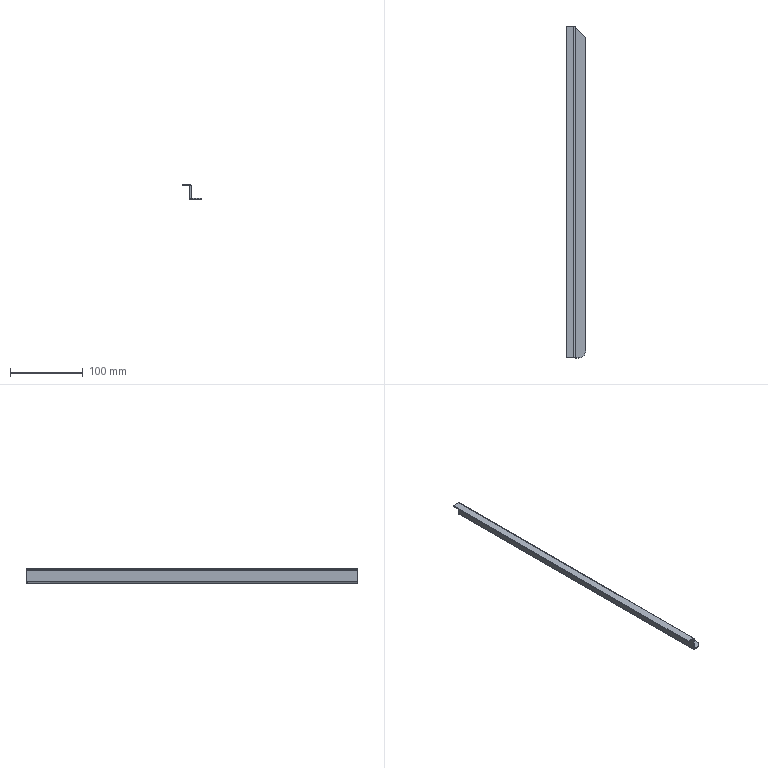Part | STEP file | Left Side Panel Frame Right | 1 solid | 21 faces | box 26.5 x 455 x 20 mm | volume 29759 mm3 | plane 14 | cylinder 7 | commonest cylinder face diameters 0.15 x2 1 x2 4 x2 20 x1
STEP:
#1=CARTESIAN_POINT('',(0.,30.962,817.654));
#2=VERTEX_POINT('',#1);
#3=CARTESIAN_POINT('',(0.,31.037,817.579));
#4=VERTEX_POINT('',#3);
#5=CARTESIAN_POINT('',(0.,30.962,817.579));
#6=DIRECTION('',(-1.,0.,0.));
#7=DIRECTION('',(0.,0.,1.));
#8=AXIS2_PLACEMENT_3D('',#5,#6,#7);
#9=CIRCLE('',#8,0.075);
#10=EDGE_CURVE('',#2,#4,#9,.T.);
#11=ORIENTED_EDGE('',*,*,#10,.F.);
#12=CARTESIAN_POINT('',(-1.5,30.962,817.654));
#13=VERTEX_POINT('',#12);
#14=CARTESIAN_POINT('',(0.,30.962,817.654));
#15=DIRECTION('',(-1.,0.,0.));
#16=VECTOR('',#15,1000.);
#17=LINE('',#14,#16);
#18=EDGE_CURVE('',#2,#13,#17,.T.);
#19=ORIENTED_EDGE('',*,*,#18,.T.);
#20=CARTESIAN_POINT('',(-1.5,31.037,817.579));
#21=VERTEX_POINT('',#20);
#22=CARTESIAN_POINT('',(-1.5,30.962,817.579));
#23=DIRECTION('',(1.,0.,0.));
#24=DIRECTION('',(0.,0.,1.));
#25=AXIS2_PLACEMENT_3D('',#22,#23,#24);
#26=CIRCLE('',#25,0.075);
#27=EDGE_CURVE('',#21,#13,#26,.T.);
#28=ORIENTED_EDGE('',*,*,#27,.F.);
#29=CARTESIAN_POINT('',(0.,31.037,817.579));
#30=DIRECTION('',(-1.,0.,0.));
#31=VECTOR('',#30,1000.);
#32=LINE('',#29,#31);
#33=EDGE_CURVE('',#4,#21,#32,.T.);
#34=ORIENTED_EDGE('',*,*,#33,.F.);
#35=EDGE_LOOP('',(#11,#19,#28,#34));
#36=FACE_OUTER_BOUND('',#35,.T.);
#37=CARTESIAN_POINT('',(0.,30.962,817.579));
#38=DIRECTION('',(-1.,0.,0.));
#39=DIRECTION('',(0.,0.,1.));
#40=AXIS2_PLACEMENT_3D('',#37,#38,#39);
#41=CYLINDRICAL_SURFACE('',#40,0.075);
#42=ADVANCED_FACE('',(#36),#41,.F.);
#43=CARTESIAN_POINT('',(-1.5,30.887,817.429));
#44=VERTEX_POINT('',#43);
#45=CARTESIAN_POINT('',(-1.5,30.887,817.579));
#46=VERTEX_POINT('',#45);
#47=CARTESIAN_POINT('',(-1.5,30.887,817.579));
#48=DIRECTION('',(0.,0.,1.));
#49=VECTOR('',#48,1000.);
#50=LINE('',#47,#49);
#51=EDGE_CURVE('',#44,#46,#50,.T.);
#52=ORIENTED_EDGE('',*,*,#51,.F.);
#53=CARTESIAN_POINT('',(-1.5,-422.413,817.429));
#54=VERTEX_POINT('',#53);
#55=CARTESIAN_POINT('',(-1.5,0.,817.429));
#56=DIRECTION('',(0.,-1.,0.));
#57=VECTOR('',#56,1000.);
#58=LINE('',#55,#57);
#59=EDGE_CURVE('',#44,#54,#58,.T.);
#60=ORIENTED_EDGE('',*,*,#59,.T.);
#61=CARTESIAN_POINT('',(-1.5,-422.413,833.429));
#62=VERTEX_POINT('',#61);
#63=CARTESIAN_POINT('',(-1.5,-422.413,0.));
#64=DIRECTION('',(0.,0.,1.));
#65=VECTOR('',#64,1000.);
#66=LINE('',#63,#65);
#67=EDGE_CURVE('',#54,#62,#66,.T.);
#68=ORIENTED_EDGE('',*,*,#67,.T.);
#69=CARTESIAN_POINT('',(-1.5,32.587,833.429));
#70=VERTEX_POINT('',#69);
#71=CARTESIAN_POINT('',(-1.5,0.,833.429));
#72=DIRECTION('',(0.,1.,0.));
#73=VECTOR('',#72,1000.);
#74=LINE('',#71,#73);
#75=EDGE_CURVE('',#62,#70,#74,.T.);
#76=ORIENTED_EDGE('',*,*,#75,.T.);
#77=CARTESIAN_POINT('',(-1.5,32.587,815.429));
#78=VERTEX_POINT('',#77);
#79=CARTESIAN_POINT('',(-1.5,32.587,0.));
#80=DIRECTION('',(0.,0.,-1.));
#81=VECTOR('',#80,1000.);
#82=LINE('',#79,#81);
#83=EDGE_CURVE('',#70,#78,#82,.T.);
#84=ORIENTED_EDGE('',*,*,#83,.T.);
#85=CARTESIAN_POINT('',(-1.5,31.037,815.429));
#86=VERTEX_POINT('',#85);
#87=CARTESIAN_POINT('',(-1.5,0.,815.429));
#88=DIRECTION('',(0.,-1.,0.));
#89=VECTOR('',#88,1000.);
#90=LINE('',#87,#89);
#91=EDGE_CURVE('',#78,#86,#90,.T.);
#92=ORIENTED_EDGE('',*,*,#91,.T.);
#93=CARTESIAN_POINT('',(-1.5,31.037,0.));
#94=DIRECTION('',(0.,0.,1.));
#95=VECTOR('',#94,1000.);
#96=LINE('',#93,#95);
#97=EDGE_CURVE('',#86,#21,#96,.T.);
#98=ORIENTED_EDGE('',*,*,#97,.T.);
#99=ORIENTED_EDGE('',*,*,#27,.T.);
#100=CARTESIAN_POINT('',(-1.5,30.962,817.579));
#101=DIRECTION('',(1.,0.,0.));
#102=DIRECTION('',(0.,0.,1.));
#103=AXIS2_PLACEMENT_3D('',#100,#101,#102);
#104=CIRCLE('',#103,0.075);
#105=EDGE_CURVE('',#13,#46,#104,.T.);
#106=ORIENTED_EDGE('',*,*,#105,.T.);
#107=EDGE_LOOP('',(#52,#60,#68,#76,#84,#92,#98,#99,#106));
#108=FACE_OUTER_BOUND('',#107,.T.);
#109=CARTESIAN_POINT('',(-1.5,0.,0.));
#110=DIRECTION('',(-1.,0.,0.));
#111=DIRECTION('',(0.,0.,1.));
#112=AXIS2_PLACEMENT_3D('',#109,#110,#111);
#113=PLANE('',#112);
#114=ADVANCED_FACE('',(#108),#113,.T.);
#115=CARTESIAN_POINT('',(0.5,-422.413,815.429));
#116=VERTEX_POINT('',#115);
#117=CARTESIAN_POINT('',(0.5,-422.413,817.429));
#118=DIRECTION('',(0.,1.,0.));
#119=DIRECTION('',(0.,0.,1.));
#120=AXIS2_PLACEMENT_3D('',#117,#118,#119);
#121=CIRCLE('',#120,2.);
#122=EDGE_CURVE('',#116,#54,#121,.T.);
#123=ORIENTED_EDGE('',*,*,#122,.T.);
#124=ORIENTED_EDGE('',*,*,#59,.F.);
#125=CARTESIAN_POINT('',(0.2,30.887,815.452));
#126=VERTEX_POINT('',#125);
#127=CARTESIAN_POINT('',(0.5,30.887,817.429));
#128=DIRECTION('',(0.,-1.,0.));
#129=DIRECTION('',(0.,0.,1.));
#130=AXIS2_PLACEMENT_3D('',#127,#128,#129);
#131=CIRCLE('',#130,2.);
#132=EDGE_CURVE('',#44,#126,#131,.T.);
#133=ORIENTED_EDGE('',*,*,#132,.T.);
#134=CARTESIAN_POINT('',(0.5,30.587,815.429));
#135=VERTEX_POINT('',#134);
#136=CARTESIAN_POINT('',(0.2,30.887,815.452));
#137=CARTESIAN_POINT('',(0.2993,30.788,815.437));
#138=CARTESIAN_POINT('',(0.3995,30.687,815.429));
#139=CARTESIAN_POINT('',(0.5,30.587,815.429));
#140=(BOUNDED_CURVE()B_SPLINE_CURVE(3,(#136,#137,#138,#139),.UNSPECIFIED.,.F.,.F.)B_SPLINE_CURVE_WITH_KNOTS((4,4),(1.42,1.571),.UNSPECIFIED.)CURVE()GEOMETRIC_REPRESENTATION_ITEM()RATIONAL_B_SPLINE_CURVE((1.,0.9981,0.9981,1.))REPRESENTATION_ITEM(''));
#141=EDGE_CURVE('',#126,#135,#140,.T.);
#142=ORIENTED_EDGE('',*,*,#141,.T.);
#143=CARTESIAN_POINT('',(0.5,30.887,815.429));
#144=DIRECTION('',(0.,-1.,0.));
#145=VECTOR('',#144,1000.);
#146=LINE('',#143,#145);
#147=EDGE_CURVE('',#135,#116,#146,.T.);
#148=ORIENTED_EDGE('',*,*,#147,.T.);
#149=EDGE_LOOP('',(#123,#124,#133,#142,#148));
#150=FACE_OUTER_BOUND('',#149,.T.);
#151=CARTESIAN_POINT('',(0.5,30.887,817.429));
#152=DIRECTION('',(0.,1.,0.));
#153=DIRECTION('',(0.,0.,1.));
#154=AXIS2_PLACEMENT_3D('',#151,#152,#153);
#155=CYLINDRICAL_SURFACE('',#154,2.);
#156=ADVANCED_FACE('',(#150),#155,.T.);
#157=CARTESIAN_POINT('',(0.,31.037,815.429));
#158=VERTEX_POINT('',#157);
#159=CARTESIAN_POINT('',(0.,31.037,815.429));
#160=DIRECTION('',(0.,0.,1.));
#161=VECTOR('',#160,1000.);
#162=LINE('',#159,#161);
#163=EDGE_CURVE('',#158,#4,#162,.T.);
#164=ORIENTED_EDGE('',*,*,#163,.T.);
#165=ORIENTED_EDGE('',*,*,#33,.T.);
#166=ORIENTED_EDGE('',*,*,#97,.F.);
#167=CARTESIAN_POINT('',(0.,31.037,815.429));
#168=DIRECTION('',(1.,0.,0.));
#169=VECTOR('',#168,1000.);
#170=LINE('',#167,#169);
#171=EDGE_CURVE('',#86,#158,#170,.T.);
#172=ORIENTED_EDGE('',*,*,#171,.T.);
#173=EDGE_LOOP('',(#164,#165,#166,#172));
#174=FACE_OUTER_BOUND('',#173,.T.);
#175=CARTESIAN_POINT('',(0.,31.037,815.429));
#176=DIRECTION('',(0.,-1.,0.));
#177=DIRECTION('',(0.,0.,-1.));
#178=AXIS2_PLACEMENT_3D('',#175,#176,#177);
#179=PLANE('',#178);
#180=ADVANCED_FACE('',(#174),#179,.T.);
#181=ORIENTED_EDGE('',*,*,#91,.F.);
#182=CARTESIAN_POINT('',(0.,32.587,815.429));
#183=VERTEX_POINT('',#182);
#184=CARTESIAN_POINT('',(-1.5,32.587,815.429));
#185=DIRECTION('',(1.,0.,0.));
#186=VECTOR('',#185,1000.);
#187=LINE('',#184,#186);
#188=EDGE_CURVE('',#78,#183,#187,.T.);
#189=ORIENTED_EDGE('',*,*,#188,.T.);
#190=CARTESIAN_POINT('',(0.,32.587,815.429));
#191=DIRECTION('',(0.,-1.,0.));
#192=VECTOR('',#191,1000.);
#193=LINE('',#190,#192);
#194=EDGE_CURVE('',#183,#158,#193,.T.);
#195=ORIENTED_EDGE('',*,*,#194,.T.);
#196=ORIENTED_EDGE('',*,*,#171,.F.);
#197=EDGE_LOOP('',(#181,#189,#195,#196));
#198=FACE_OUTER_BOUND('',#197,.T.);
#199=CARTESIAN_POINT('',(-1.5,32.587,815.429));
#200=DIRECTION('',(0.,0.,-1.));
#201=DIRECTION('',(0.,1.,0.));
#202=AXIS2_PLACEMENT_3D('',#199,#200,#201);
#203=PLANE('',#202);
#204=ADVANCED_FACE('',(#198),#203,.T.);
#205=CARTESIAN_POINT('',(0.,32.587,833.429));
#206=VERTEX_POINT('',#205);
#207=CARTESIAN_POINT('',(0.,32.587,835.429));
#208=DIRECTION('',(0.,0.,-1.));
#209=VECTOR('',#208,1000.);
#210=LINE('',#207,#209);
#211=EDGE_CURVE('',#206,#183,#210,.T.);
#212=ORIENTED_EDGE('',*,*,#211,.T.);
#213=ORIENTED_EDGE('',*,*,#188,.F.);
#214=ORIENTED_EDGE('',*,*,#83,.F.);
#215=CARTESIAN_POINT('',(-2.,32.587,833.929));
#216=VERTEX_POINT('',#215);
#217=CARTESIAN_POINT('',(-2.,32.587,833.429));
#218=DIRECTION('',(0.,1.,0.));
#219=DIRECTION('',(0.,0.,1.));
#220=AXIS2_PLACEMENT_3D('',#217,#218,#219);
#221=CIRCLE('',#220,0.5);
#222=EDGE_CURVE('',#216,#70,#221,.T.);
#223=ORIENTED_EDGE('',*,*,#222,.F.);
#224=CARTESIAN_POINT('',(-12.,32.587,833.929));
#225=VERTEX_POINT('',#224);
#226=CARTESIAN_POINT('',(0.,32.587,833.929));
#227=DIRECTION('',(1.,0.,0.));
#228=VECTOR('',#227,1000.);
#229=LINE('',#226,#228);
#230=EDGE_CURVE('',#225,#216,#229,.T.);
#231=ORIENTED_EDGE('',*,*,#230,.F.);
#232=CARTESIAN_POINT('',(-12.,32.587,835.429));
#233=VERTEX_POINT('',#232);
#234=CARTESIAN_POINT('',(-12.,32.587,835.429));
#235=DIRECTION('',(0.,0.,1.));
#236=VECTOR('',#235,1000.);
#237=LINE('',#234,#236);
#238=EDGE_CURVE('',#225,#233,#237,.T.);
#239=ORIENTED_EDGE('',*,*,#238,.T.);
#240=CARTESIAN_POINT('',(-2.,32.587,835.429));
#241=VERTEX_POINT('',#240);
#242=CARTESIAN_POINT('',(-12.,32.587,835.429));
#243=DIRECTION('',(-1.,0.,0.));
#244=VECTOR('',#243,1000.);
#245=LINE('',#242,#244);
#246=EDGE_CURVE('',#241,#233,#245,.T.);
#247=ORIENTED_EDGE('',*,*,#246,.F.);
#248=CARTESIAN_POINT('',(-2.,32.587,833.429));
#249=DIRECTION('',(0.,-1.,0.));
#250=DIRECTION('',(0.,0.,1.));
#251=AXIS2_PLACEMENT_3D('',#248,#249,#250);
#252=CIRCLE('',#251,2.);
#253=EDGE_CURVE('',#206,#241,#252,.T.);
#254=ORIENTED_EDGE('',*,*,#253,.F.);
#255=EDGE_LOOP('',(#212,#213,#214,#223,#231,#239,#247,#254));
#256=FACE_OUTER_BOUND('',#255,.T.);
#257=CARTESIAN_POINT('',(-1.5,32.587,835.429));
#258=DIRECTION('',(0.,1.,0.));
#259=DIRECTION('',(0.,0.,1.));
#260=AXIS2_PLACEMENT_3D('',#257,#258,#259);
#261=PLANE('',#260);
#262=ADVANCED_FACE('',(#256),#261,.T.);
#263=CARTESIAN_POINT('',(-2.,-422.413,833.929));
#264=VERTEX_POINT('',#263);
#265=CARTESIAN_POINT('',(-2.,-422.413,833.429));
#266=DIRECTION('',(0.,1.,0.));
#267=DIRECTION('',(0.,0.,1.));
#268=AXIS2_PLACEMENT_3D('',#265,#266,#267);
#269=CIRCLE('',#268,0.5);
#270=EDGE_CURVE('',#264,#62,#269,.T.);
#271=ORIENTED_EDGE('',*,*,#270,.F.);
#272=CARTESIAN_POINT('',(-2.,32.587,833.929));
#273=DIRECTION('',(0.,-1.,0.));
#274=VECTOR('',#273,1000.);
#275=LINE('',#272,#274);
#276=EDGE_CURVE('',#216,#264,#275,.T.);
#277=ORIENTED_EDGE('',*,*,#276,.F.);
#278=ORIENTED_EDGE('',*,*,#222,.T.);
#279=ORIENTED_EDGE('',*,*,#75,.F.);
#280=EDGE_LOOP('',(#271,#277,#278,#279));
#281=FACE_OUTER_BOUND('',#280,.T.);
#282=CARTESIAN_POINT('',(-2.,32.587,833.429));
#283=DIRECTION('',(0.,1.,0.));
#284=DIRECTION('',(0.,0.,1.));
#285=AXIS2_PLACEMENT_3D('',#282,#283,#284);
#286=CYLINDRICAL_SURFACE('',#285,0.5);
#287=ADVANCED_FACE('',(#281),#286,.F.);
#288=ORIENTED_EDGE('',*,*,#67,.F.);
#289=ORIENTED_EDGE('',*,*,#122,.F.);
#290=CARTESIAN_POINT('',(4.5,-422.413,815.429));
#291=VERTEX_POINT('',#290);
#292=CARTESIAN_POINT('',(0.,-422.413,815.429));
#293=DIRECTION('',(1.,0.,0.));
#294=VECTOR('',#293,1000.);
#295=LINE('',#292,#294);
#296=EDGE_CURVE('',#116,#291,#295,.T.);
#297=ORIENTED_EDGE('',*,*,#296,.T.);
#298=CARTESIAN_POINT('',(4.5,-422.413,816.929));
#299=VERTEX_POINT('',#298);
#300=CARTESIAN_POINT('',(4.5,-422.413,815.429));
#301=DIRECTION('',(0.,0.,-1.));
#302=VECTOR('',#301,1000.);
#303=LINE('',#300,#302);
#304=EDGE_CURVE('',#299,#291,#303,.T.);
#305=ORIENTED_EDGE('',*,*,#304,.F.);
#306=CARTESIAN_POINT('',(0.5,-422.413,816.929));
#307=VERTEX_POINT('',#306);
#308=CARTESIAN_POINT('',(0.,-422.413,816.929));
#309=DIRECTION('',(1.,0.,0.));
#310=VECTOR('',#309,1000.);
#311=LINE('',#308,#310);
#312=EDGE_CURVE('',#307,#299,#311,.T.);
#313=ORIENTED_EDGE('',*,*,#312,.F.);
#314=CARTESIAN_POINT('',(0.,-422.413,817.429));
#315=VERTEX_POINT('',#314);
#316=CARTESIAN_POINT('',(0.5,-422.413,817.429));
#317=DIRECTION('',(0.,1.,0.));
#318=DIRECTION('',(0.,0.,1.));
#319=AXIS2_PLACEMENT_3D('',#316,#317,#318);
#320=CIRCLE('',#319,0.5);
#321=EDGE_CURVE('',#307,#315,#320,.T.);
#322=ORIENTED_EDGE('',*,*,#321,.T.);
#323=CARTESIAN_POINT('',(0.,-422.413,833.429));
#324=VERTEX_POINT('',#323);
#325=CARTESIAN_POINT('',(0.,-422.413,815.429));
#326=DIRECTION('',(0.,0.,1.));
#327=VECTOR('',#326,1000.);
#328=LINE('',#325,#327);
#329=EDGE_CURVE('',#315,#324,#328,.T.);
#330=ORIENTED_EDGE('',*,*,#329,.T.);
#331=CARTESIAN_POINT('',(-2.,-422.413,835.429));
#332=VERTEX_POINT('',#331);
#333=CARTESIAN_POINT('',(-2.,-422.413,833.429));
#334=DIRECTION('',(0.,1.,0.));
#335=DIRECTION('',(0.,0.,1.));
#336=AXIS2_PLACEMENT_3D('',#333,#334,#335);
#337=CIRCLE('',#336,2.);
#338=EDGE_CURVE('',#332,#324,#337,.T.);
#339=ORIENTED_EDGE('',*,*,#338,.F.);
#340=CARTESIAN_POINT('',(-12.,-422.413,835.429));
#341=VERTEX_POINT('',#340);
#342=CARTESIAN_POINT('',(-1.5,-422.413,835.429));
#343=DIRECTION('',(1.,0.,0.));
#344=VECTOR('',#343,1000.);
#345=LINE('',#342,#344);
#346=EDGE_CURVE('',#341,#332,#345,.T.);
#347=ORIENTED_EDGE('',*,*,#346,.F.);
#348=CARTESIAN_POINT('',(-12.,-422.413,833.929));
#349=VERTEX_POINT('',#348);
#350=CARTESIAN_POINT('',(-12.,-422.413,835.429));
#351=DIRECTION('',(0.,0.,-1.));
#352=VECTOR('',#351,1000.);
#353=LINE('',#350,#352);
#354=EDGE_CURVE('',#341,#349,#353,.T.);
#355=ORIENTED_EDGE('',*,*,#354,.T.);
#356=CARTESIAN_POINT('',(0.,-422.413,833.929));
#357=DIRECTION('',(-1.,0.,0.));
#358=VECTOR('',#357,1000.);
#359=LINE('',#356,#358);
#360=EDGE_CURVE('',#264,#349,#359,.T.);
#361=ORIENTED_EDGE('',*,*,#360,.F.);
#362=ORIENTED_EDGE('',*,*,#270,.T.);
#363=EDGE_LOOP('',(#288,#289,#297,#305,#313,#322,#330,#339,#347,#355,#361,#362));
#364=FACE_OUTER_BOUND('',#363,.T.);
#365=CARTESIAN_POINT('',(-1.5,-422.413,815.429));
#366=DIRECTION('',(0.,-1.,0.));
#367=DIRECTION('',(0.,0.,-1.));
#368=AXIS2_PLACEMENT_3D('',#365,#366,#367);
#369=PLANE('',#368);
#370=ADVANCED_FACE('',(#364),#369,.T.);
#371=CARTESIAN_POINT('',(14.5,-412.413,815.429));
#372=VERTEX_POINT('',#371);
#373=CARTESIAN_POINT('',(4.5,-412.413,815.429));
#374=DIRECTION('',(0.,0.,1.));
#375=DIRECTION('',(1.,0.,0.));
#376=AXIS2_PLACEMENT_3D('',#373,#374,#375);
#377=CIRCLE('',#376,10.);
#378=EDGE_CURVE('',#291,#372,#377,.T.);
#379=ORIENTED_EDGE('',*,*,#378,.F.);
#380=ORIENTED_EDGE('',*,*,#296,.F.);
#381=ORIENTED_EDGE('',*,*,#147,.F.);
#382=CARTESIAN_POINT('',(14.5,16.587,815.429));
#383=VERTEX_POINT('',#382);
#384=CARTESIAN_POINT('',(14.5,16.587,815.429));
#385=DIRECTION('',(-0.7071,0.7071,0.));
#386=VECTOR('',#385,1000.);
#387=LINE('',#384,#386);
#388=EDGE_CURVE('',#383,#135,#387,.T.);
#389=ORIENTED_EDGE('',*,*,#388,.F.);
#390=CARTESIAN_POINT('',(14.5,0.,815.429));
#391=DIRECTION('',(0.,1.,0.));
#392=VECTOR('',#391,1000.);
#393=LINE('',#390,#392);
#394=EDGE_CURVE('',#372,#383,#393,.T.);
#395=ORIENTED_EDGE('',*,*,#394,.F.);
#396=EDGE_LOOP('',(#379,#380,#381,#389,#395));
#397=FACE_OUTER_BOUND('',#396,.T.);
#398=CARTESIAN_POINT('',(0.,0.,815.429));
#399=DIRECTION('',(0.,0.,1.));
#400=DIRECTION('',(0.,-1.,0.));
#401=AXIS2_PLACEMENT_3D('',#398,#399,#400);
#402=PLANE('',#401);
#403=ADVANCED_FACE('',(#397),#402,.F.);
#404=CARTESIAN_POINT('',(0.2,30.887,817.029));
#405=VERTEX_POINT('',#404);
#406=CARTESIAN_POINT('',(0.2,30.887,817.429));
#407=DIRECTION('',(0.,0.,1.));
#408=VECTOR('',#407,1000.);
#409=LINE('',#406,#408);
#410=EDGE_CURVE('',#126,#405,#409,.T.);
#411=ORIENTED_EDGE('',*,*,#410,.F.);
#412=ORIENTED_EDGE('',*,*,#132,.F.);
#413=ORIENTED_EDGE('',*,*,#51,.T.);
#414=CARTESIAN_POINT('',(0.,30.887,817.579));
#415=VERTEX_POINT('',#414);
#416=CARTESIAN_POINT('',(0.,30.887,817.579));
#417=DIRECTION('',(1.,0.,0.));
#418=VECTOR('',#417,1000.);
#419=LINE('',#416,#418);
#420=EDGE_CURVE('',#46,#415,#419,.T.);
#421=ORIENTED_EDGE('',*,*,#420,.T.);
#422=CARTESIAN_POINT('',(0.,30.887,817.429));
#423=VERTEX_POINT('',#422);
#424=CARTESIAN_POINT('',(0.,30.887,0.));
#425=DIRECTION('',(0.,0.,-1.));
#426=VECTOR('',#425,1000.);
#427=LINE('',#424,#426);
#428=EDGE_CURVE('',#415,#423,#427,.T.);
#429=ORIENTED_EDGE('',*,*,#428,.T.);
#430=CARTESIAN_POINT('',(0.5,30.887,817.429));
#431=DIRECTION('',(0.,-1.,0.));
#432=DIRECTION('',(0.,0.,1.));
#433=AXIS2_PLACEMENT_3D('',#430,#431,#432);
#434=CIRCLE('',#433,0.5);
#435=EDGE_CURVE('',#423,#405,#434,.T.);
#436=ORIENTED_EDGE('',*,*,#435,.T.);
#437=EDGE_LOOP('',(#411,#412,#413,#421,#429,#436));
#438=FACE_OUTER_BOUND('',#437,.T.);
#439=CARTESIAN_POINT('',(0.5,30.887,817.429));
#440=DIRECTION('',(0.,-1.,0.));
#441=DIRECTION('',(0.,0.,-1.));
#442=AXIS2_PLACEMENT_3D('',#439,#440,#441);
#443=PLANE('',#442);
#444=ADVANCED_FACE('',(#438),#443,.F.);
#445=ORIENTED_EDGE('',*,*,#18,.F.);
#446=CARTESIAN_POINT('',(0.,30.962,817.579));
#447=DIRECTION('',(-1.,0.,0.));
#448=DIRECTION('',(0.,0.,1.));
#449=AXIS2_PLACEMENT_3D('',#446,#447,#448);
#450=CIRCLE('',#449,0.075);
#451=EDGE_CURVE('',#415,#2,#450,.T.);
#452=ORIENTED_EDGE('',*,*,#451,.F.);
#453=ORIENTED_EDGE('',*,*,#420,.F.);
#454=ORIENTED_EDGE('',*,*,#105,.F.);
#455=EDGE_LOOP('',(#445,#452,#453,#454));
#456=FACE_OUTER_BOUND('',#455,.T.);
#457=CARTESIAN_POINT('',(0.,30.962,817.579));
#458=DIRECTION('',(-1.,0.,0.));
#459=DIRECTION('',(0.,0.,1.));
#460=AXIS2_PLACEMENT_3D('',#457,#458,#459);
#461=CYLINDRICAL_SURFACE('',#460,0.075);
#462=ADVANCED_FACE('',(#456),#461,.F.);
#463=ORIENTED_EDGE('',*,*,#329,.F.);
#464=CARTESIAN_POINT('',(0.,0.,817.429));
#465=DIRECTION('',(0.,-1.,0.));
#466=VECTOR('',#465,1000.);
#467=LINE('',#464,#466);
#468=EDGE_CURVE('',#423,#315,#467,.T.);
#469=ORIENTED_EDGE('',*,*,#468,.F.);
#470=ORIENTED_EDGE('',*,*,#428,.F.);
#471=ORIENTED_EDGE('',*,*,#451,.T.);
#472=ORIENTED_EDGE('',*,*,#10,.T.);
#473=ORIENTED_EDGE('',*,*,#163,.F.);
#474=ORIENTED_EDGE('',*,*,#194,.F.);
#475=ORIENTED_EDGE('',*,*,#211,.F.);
#476=CARTESIAN_POINT('',(0.,0.,833.429));
#477=DIRECTION('',(0.,1.,0.));
#478=VECTOR('',#477,1000.);
#479=LINE('',#476,#478);
#480=EDGE_CURVE('',#324,#206,#479,.T.);
#481=ORIENTED_EDGE('',*,*,#480,.F.);
#482=EDGE_LOOP('',(#463,#469,#470,#471,#472,#473,#474,#475,#481));
#483=FACE_OUTER_BOUND('',#482,.T.);
#484=CARTESIAN_POINT('',(0.,0.,0.));
#485=DIRECTION('',(-1.,0.,0.));
#486=DIRECTION('',(0.,0.,1.));
#487=AXIS2_PLACEMENT_3D('',#484,#485,#486);
#488=PLANE('',#487);
#489=ADVANCED_FACE('',(#483),#488,.F.);
#490=ORIENTED_EDGE('',*,*,#360,.T.);
#491=CARTESIAN_POINT('',(-12.,0.,833.929));
#492=DIRECTION('',(0.,1.,0.));
#493=VECTOR('',#492,1000.);
#494=LINE('',#491,#493);
#495=EDGE_CURVE('',#349,#225,#494,.T.);
#496=ORIENTED_EDGE('',*,*,#495,.T.);
#497=ORIENTED_EDGE('',*,*,#230,.T.);
#498=ORIENTED_EDGE('',*,*,#276,.T.);
#499=EDGE_LOOP('',(#490,#496,#497,#498));
#500=FACE_OUTER_BOUND('',#499,.T.);
#501=CARTESIAN_POINT('',(0.,0.,833.929));
#502=DIRECTION('',(0.,0.,-1.));
#503=DIRECTION('',(-1.,0.,0.));
#504=AXIS2_PLACEMENT_3D('',#501,#502,#503);
#505=PLANE('',#504);
#506=ADVANCED_FACE('',(#500),#505,.T.);
#507=CARTESIAN_POINT('',(14.5,-412.413,816.929));
#508=VERTEX_POINT('',#507);
#509=CARTESIAN_POINT('',(14.5,-412.413,815.429));
#510=DIRECTION('',(0.,0.,1.));
#511=VECTOR('',#510,1000.);
#512=LINE('',#509,#511);
#513=EDGE_CURVE('',#372,#508,#512,.T.);
#514=ORIENTED_EDGE('',*,*,#513,.F.);
#515=ORIENTED_EDGE('',*,*,#394,.T.);
#516=CARTESIAN_POINT('',(14.5,16.587,816.929));
#517=VERTEX_POINT('',#516);
#518=CARTESIAN_POINT('',(14.5,16.587,815.429));
#519=DIRECTION('',(0.,0.,-1.));
#520=VECTOR('',#519,1000.);
#521=LINE('',#518,#520);
#522=EDGE_CURVE('',#517,#383,#521,.T.);
#523=ORIENTED_EDGE('',*,*,#522,.F.);
#524=CARTESIAN_POINT('',(14.5,-422.413,816.929));
#525=DIRECTION('',(0.,1.,0.));
#526=VECTOR('',#525,1000.);
#527=LINE('',#524,#526);
#528=EDGE_CURVE('',#508,#517,#527,.T.);
#529=ORIENTED_EDGE('',*,*,#528,.F.);
#530=EDGE_LOOP('',(#514,#515,#523,#529));
#531=FACE_OUTER_BOUND('',#530,.T.);
#532=CARTESIAN_POINT('',(14.5,-422.413,815.429));
#533=DIRECTION('',(-1.,0.,0.));
#534=DIRECTION('',(0.,0.,1.));
#535=AXIS2_PLACEMENT_3D('',#532,#533,#534);
#536=PLANE('',#535);
#537=ADVANCED_FACE('',(#531),#536,.F.);
#538=CARTESIAN_POINT('',(4.5,-412.413,816.929));
#539=DIRECTION('',(0.,0.,-1.));
#540=DIRECTION('',(1.,0.,0.));
#541=AXIS2_PLACEMENT_3D('',#538,#539,#540);
#542=CIRCLE('',#541,10.);
#543=EDGE_CURVE('',#508,#299,#542,.T.);
#544=ORIENTED_EDGE('',*,*,#543,.T.);
#545=ORIENTED_EDGE('',*,*,#304,.T.);
#546=ORIENTED_EDGE('',*,*,#378,.T.);
#547=ORIENTED_EDGE('',*,*,#513,.T.);
#548=EDGE_LOOP('',(#544,#545,#546,#547));
#549=FACE_OUTER_BOUND('',#548,.T.);
#550=CARTESIAN_POINT('',(4.5,-412.413,815.429));
#551=DIRECTION('',(0.,0.,1.));
#552=DIRECTION('',(1.,0.,0.));
#553=AXIS2_PLACEMENT_3D('',#550,#551,#552);
#554=CYLINDRICAL_SURFACE('',#553,10.);
#555=ADVANCED_FACE('',(#549),#554,.T.);
#556=ORIENTED_EDGE('',*,*,#410,.T.);
#557=CARTESIAN_POINT('',(0.5,30.587,816.929));
#558=VERTEX_POINT('',#557);
#559=CARTESIAN_POINT('',(0.5,30.587,816.929));
#560=CARTESIAN_POINT('',(0.3909,30.696,816.929));
#561=CARTESIAN_POINT('',(0.2873,30.8,816.964));
#562=CARTESIAN_POINT('',(0.2,30.887,817.029));
#563=(BOUNDED_CURVE()B_SPLINE_CURVE(3,(#559,#560,#561,#562),.UNSPECIFIED.,.F.,.F.)B_SPLINE_CURVE_WITH_KNOTS((4,4),(4.712,5.356),.UNSPECIFIED.)CURVE()GEOMETRIC_REPRESENTATION_ITEM()RATIONAL_B_SPLINE_CURVE((1.,0.9658,0.9658,1.))REPRESENTATION_ITEM(''));
#564=EDGE_CURVE('',#558,#405,#563,.T.);
#565=ORIENTED_EDGE('',*,*,#564,.F.);
#566=CARTESIAN_POINT('',(14.5,16.587,816.929));
#567=DIRECTION('',(-0.7071,0.7071,0.));
#568=VECTOR('',#567,1000.);
#569=LINE('',#566,#568);
#570=EDGE_CURVE('',#517,#558,#569,.T.);
#571=ORIENTED_EDGE('',*,*,#570,.F.);
#572=ORIENTED_EDGE('',*,*,#522,.T.);
#573=ORIENTED_EDGE('',*,*,#388,.T.);
#574=ORIENTED_EDGE('',*,*,#141,.F.);
#575=EDGE_LOOP('',(#556,#565,#571,#572,#573,#574));
#576=FACE_OUTER_BOUND('',#575,.T.);
#577=CARTESIAN_POINT('',(14.5,16.587,815.429));
#578=DIRECTION('',(-0.7071,-0.7071,0.));
#579=DIRECTION('',(0.7071,-0.7071,0.));
#580=AXIS2_PLACEMENT_3D('',#577,#578,#579);
#581=PLANE('',#580);
#582=ADVANCED_FACE('',(#576),#581,.F.);
#583=CARTESIAN_POINT('',(-2.,32.587,835.429));
#584=DIRECTION('',(0.,-1.,0.));
#585=VECTOR('',#584,1000.);
#586=LINE('',#583,#585);
#587=EDGE_CURVE('',#241,#332,#586,.T.);
#588=ORIENTED_EDGE('',*,*,#587,.T.);
#589=ORIENTED_EDGE('',*,*,#338,.T.);
#590=ORIENTED_EDGE('',*,*,#480,.T.);
#591=ORIENTED_EDGE('',*,*,#253,.T.);
#592=EDGE_LOOP('',(#588,#589,#590,#591));
#593=FACE_OUTER_BOUND('',#592,.T.);
#594=CARTESIAN_POINT('',(-2.,32.587,833.429));
#595=DIRECTION('',(0.,1.,0.));
#596=DIRECTION('',(0.,0.,1.));
#597=AXIS2_PLACEMENT_3D('',#594,#595,#596);
#598=CYLINDRICAL_SURFACE('',#597,2.);
#599=ADVANCED_FACE('',(#593),#598,.T.);
#600=ORIENTED_EDGE('',*,*,#564,.T.);
#601=ORIENTED_EDGE('',*,*,#435,.F.);
#602=ORIENTED_EDGE('',*,*,#468,.T.);
#603=ORIENTED_EDGE('',*,*,#321,.F.);
#604=CARTESIAN_POINT('',(0.5,30.887,816.929));
#605=DIRECTION('',(0.,-1.,0.));
#606=VECTOR('',#605,1000.);
#607=LINE('',#604,#606);
#608=EDGE_CURVE('',#558,#307,#607,.T.);
#609=ORIENTED_EDGE('',*,*,#608,.F.);
#610=EDGE_LOOP('',(#600,#601,#602,#603,#609));
#611=FACE_OUTER_BOUND('',#610,.T.);
#612=CARTESIAN_POINT('',(0.5,30.887,817.429));
#613=DIRECTION('',(0.,1.,0.));
#614=DIRECTION('',(0.,0.,1.));
#615=AXIS2_PLACEMENT_3D('',#612,#613,#614);
#616=CYLINDRICAL_SURFACE('',#615,0.5);
#617=ADVANCED_FACE('',(#611),#616,.F.);
#618=ORIENTED_EDGE('',*,*,#354,.F.);
#619=CARTESIAN_POINT('',(-12.,-422.413,835.429));
#620=DIRECTION('',(0.,-1.,0.));
#621=VECTOR('',#620,1000.);
#622=LINE('',#619,#621);
#623=EDGE_CURVE('',#233,#341,#622,.T.);
#624=ORIENTED_EDGE('',*,*,#623,.F.);
#625=ORIENTED_EDGE('',*,*,#238,.F.);
#626=ORIENTED_EDGE('',*,*,#495,.F.);
#627=EDGE_LOOP('',(#618,#624,#625,#626));
#628=FACE_OUTER_BOUND('',#627,.T.);
#629=CARTESIAN_POINT('',(-12.,-422.413,835.429));
#630=DIRECTION('',(1.,0.,0.));
#631=DIRECTION('',(0.,0.,-1.));
#632=AXIS2_PLACEMENT_3D('',#629,#630,#631);
#633=PLANE('',#632);
#634=ADVANCED_FACE('',(#628),#633,.F.);
#635=ORIENTED_EDGE('',*,*,#570,.T.);
#636=ORIENTED_EDGE('',*,*,#608,.T.);
#637=ORIENTED_EDGE('',*,*,#312,.T.);
#638=ORIENTED_EDGE('',*,*,#543,.F.);
#639=ORIENTED_EDGE('',*,*,#528,.T.);
#640=EDGE_LOOP('',(#635,#636,#637,#638,#639));
#641=FACE_OUTER_BOUND('',#640,.T.);
#642=CARTESIAN_POINT('',(0.,0.,816.929));
#643=DIRECTION('',(0.,0.,1.));
#644=DIRECTION('',(0.,-1.,0.));
#645=AXIS2_PLACEMENT_3D('',#642,#643,#644);
#646=PLANE('',#645);
#647=ADVANCED_FACE('',(#641),#646,.T.);
#648=ORIENTED_EDGE('',*,*,#246,.T.);
#649=ORIENTED_EDGE('',*,*,#623,.T.);
#650=ORIENTED_EDGE('',*,*,#346,.T.);
#651=ORIENTED_EDGE('',*,*,#587,.F.);
#652=EDGE_LOOP('',(#648,#649,#650,#651));
#653=FACE_OUTER_BOUND('',#652,.T.);
#654=CARTESIAN_POINT('',(0.,0.,835.429));
#655=DIRECTION('',(0.,0.,-1.));
#656=DIRECTION('',(-1.,0.,0.));
#657=AXIS2_PLACEMENT_3D('',#654,#655,#656);
#658=PLANE('',#657);
#659=ADVANCED_FACE('',(#653),#658,.F.);
#660=CLOSED_SHELL('',(#42,#114,#156,#180,#204,#262,#287,#370,#403,#444,#462,#489,#506,#537,#555,#582,#599,#617,#634,#647,#659));
#661=MANIFOLD_SOLID_BREP('',#660);
#662=CARTESIAN_POINT('',(0.,0.,0.));
#663=DIRECTION('',(0.,0.,1.));
#664=DIRECTION('',(1.,0.,0.));
#665=AXIS2_PLACEMENT_3D('',#662,#663,#664);
#666=(LENGTH_UNIT()NAMED_UNIT(*)SI_UNIT(.MILLI.,.METRE.));
#667=UNCERTAINTY_MEASURE_WITH_UNIT(LENGTH_MEASURE(0.00001),#666,'','');
#668=(NAMED_UNIT(*)PLANE_ANGLE_UNIT()SI_UNIT($,.RADIAN.));
#669=(NAMED_UNIT(*)SI_UNIT($,.STERADIAN.)SOLID_ANGLE_UNIT());
#670=(GEOMETRIC_REPRESENTATION_CONTEXT(3)GLOBAL_UNCERTAINTY_ASSIGNED_CONTEXT((#667))GLOBAL_UNIT_ASSIGNED_CONTEXT((#666,#668,#669))REPRESENTATION_CONTEXT('',''));
#671=ADVANCED_BREP_SHAPE_REPRESENTATION('',(#661,#665),#670);